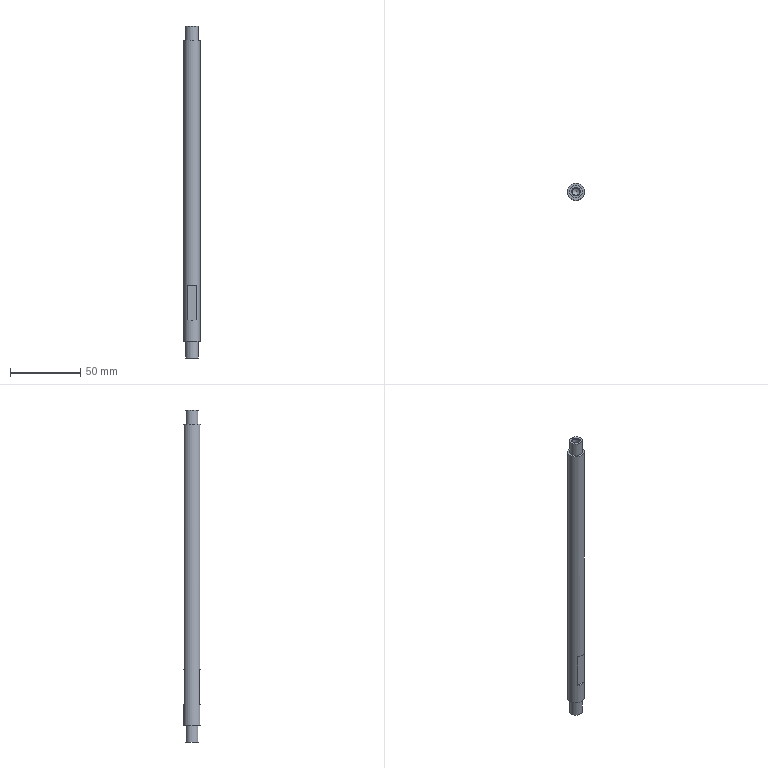Part | STEP file | YBQDJ-YY-10 | 1 solid | 19 faces | box 12 x 12 x 237 mm | volume 24995 mm3 | plane 10 | cylinder 5 | cone 4 | commonest cylinder face diameters 5 x2 9 x2 12 x1
STEP:
#1=CARTESIAN_POINT('',(0.,0.,0.));
#2=DIRECTION('',(0.,0.,1.));
#3=DIRECTION('',(1.,0.,0.));
#4=AXIS2_PLACEMENT_3D('',#1,#2,#3);
#5=CARTESIAN_POINT('',(260.5,385.,235.));
#6=VERTEX_POINT('',#5);
#7=CARTESIAN_POINT('',(266.5,385.,235.));
#8=DIRECTION('',(0.,0.,1.));
#9=DIRECTION('',(-1.,0.,0.));
#10=AXIS2_PLACEMENT_3D('',#7,#8,#9);
#11=CIRCLE('',#10,6.);
#12=CARTESIAN_POINT('',(266.5,385.,220.));
#13=DIRECTION('',(0.,0.,-1.));
#14=DIRECTION('',(1.,0.,0.));
#15=AXIS2_PLACEMENT_3D('',#12,#13,#14);
#16=CYLINDRICAL_SURFACE('',#15,6.);
#17=CARTESIAN_POINT('',(9.425,-15.));
#18=DIRECTION('',(-1.,0.));
#19=VECTOR('',#18,1.);
#20=LINE('',#17,#19);
#21=(GEOMETRIC_REPRESENTATION_CONTEXT(2)PARAMETRIC_REPRESENTATION_CONTEXT()REPRESENTATION_CONTEXT('',''));
#22=DEFINITIONAL_REPRESENTATION('',(#20),#21);
#23=PCURVE('',#16,#22);
#24=CARTESIAN_POINT('',(547.497,775.,235.));
#25=DIRECTION('',(0.,0.,1.));
#26=DIRECTION('',(-1.,0.,0.));
#27=AXIS2_PLACEMENT_3D('',#24,#25,#26);
#28=PLANE('',#27);
#29=CARTESIAN_POINT('',(280.997,390.));
#30=DIRECTION('',(1.,0.));
#31=AXIS2_PLACEMENT_2D('',#29,#30);
#32=CIRCLE('',#31,6.);
#33=(GEOMETRIC_REPRESENTATION_CONTEXT(2)PARAMETRIC_REPRESENTATION_CONTEXT()REPRESENTATION_CONTEXT('',''));
#34=DEFINITIONAL_REPRESENTATION('',(#32),#33);
#35=PCURVE('',#28,#34);
#36=SURFACE_CURVE('',#11,(#23,#35),.PCURVE_S1.);
#37=EDGE_CURVE('',#6,#6,#36,.T.);
#38=ORIENTED_EDGE('',*,*,#37,.F.);
#39=CARTESIAN_POINT('',(260.5,385.,20.));
#40=VERTEX_POINT('',#39);
#41=CARTESIAN_POINT('',(260.5,385.,235.));
#42=CARTESIAN_POINT('',(260.5,385.,20.));
#43=B_SPLINE_CURVE_WITH_KNOTS('',1,(#41,#42),.UNSPECIFIED.,.F.,.F.,(2,2),(-15.,200.),.PIECEWISE_BEZIER_KNOTS.);
#44=CARTESIAN_POINT('',(9.425,0.));
#45=DIRECTION('',(0.,1.));
#46=VECTOR('',#45,1.);
#47=LINE('',#44,#46);
#48=(GEOMETRIC_REPRESENTATION_CONTEXT(2)PARAMETRIC_REPRESENTATION_CONTEXT()REPRESENTATION_CONTEXT('',''));
#49=DEFINITIONAL_REPRESENTATION('',(#47),#48);
#50=PCURVE('',#16,#49);
#51=CARTESIAN_POINT('',(3.142,0.));
#52=DIRECTION('',(0.,1.));
#53=VECTOR('',#52,1.);
#54=LINE('',#51,#53);
#55=(GEOMETRIC_REPRESENTATION_CONTEXT(2)PARAMETRIC_REPRESENTATION_CONTEXT()REPRESENTATION_CONTEXT('',''));
#56=DEFINITIONAL_REPRESENTATION('',(#54),#55);
#57=PCURVE('',#16,#56);
#58=SEAM_CURVE('',#43,(#50,#57),.PCURVE_S1.);
#59=EDGE_CURVE('',#6,#40,#58,.T.);
#60=ORIENTED_EDGE('',*,*,#59,.T.);
#61=CARTESIAN_POINT('',(266.5,385.,20.));
#62=DIRECTION('',(0.,0.,1.));
#63=DIRECTION('',(-1.,0.,0.));
#64=AXIS2_PLACEMENT_3D('',#61,#62,#63);
#65=CIRCLE('',#64,6.);
#66=CARTESIAN_POINT('',(9.425,200.));
#67=DIRECTION('',(-1.,0.));
#68=VECTOR('',#67,1.);
#69=LINE('',#66,#68);
#70=(GEOMETRIC_REPRESENTATION_CONTEXT(2)PARAMETRIC_REPRESENTATION_CONTEXT()REPRESENTATION_CONTEXT('',''));
#71=DEFINITIONAL_REPRESENTATION('',(#69),#70);
#72=PCURVE('',#16,#71);
#73=CARTESIAN_POINT('',(266.5,385.,20.));
#74=DIRECTION('',(0.,0.,1.));
#75=DIRECTION('',(-1.,0.,0.));
#76=AXIS2_PLACEMENT_3D('',#73,#74,#75);
#77=PLANE('',#76);
#78=CARTESIAN_POINT('',(0.,0.));
#79=DIRECTION('',(1.,0.));
#80=AXIS2_PLACEMENT_2D('',#78,#79);
#81=CIRCLE('',#80,6.);
#82=(GEOMETRIC_REPRESENTATION_CONTEXT(2)PARAMETRIC_REPRESENTATION_CONTEXT()REPRESENTATION_CONTEXT('',''));
#83=DEFINITIONAL_REPRESENTATION('',(#81),#82);
#84=PCURVE('',#77,#83);
#85=SURFACE_CURVE('',#65,(#72,#84),.PCURVE_S1.);
#86=EDGE_CURVE('',#40,#40,#85,.T.);
#87=ORIENTED_EDGE('',*,*,#86,.T.);
#88=ORIENTED_EDGE('',*,*,#59,.F.);
#89=EDGE_LOOP('',(#38,#60,#87,#88));
#90=FACE_BOUND('',#89,.T.);
#91=CARTESIAN_POINT('',(263.183,390.,60.));
#92=VERTEX_POINT('',#91);
#93=CARTESIAN_POINT('',(269.817,390.,60.));
#94=VERTEX_POINT('',#93);
#95=CARTESIAN_POINT('',(266.5,385.,60.));
#96=DIRECTION('',(0.,0.,-1.));
#97=DIRECTION('',(0.,1.,0.));
#98=AXIS2_PLACEMENT_3D('',#95,#96,#97);
#99=CIRCLE('',#98,6.);
#100=CARTESIAN_POINT('',(-1.571,160.));
#101=DIRECTION('',(1.,0.));
#102=VECTOR('',#101,1.);
#103=LINE('',#100,#102);
#104=(GEOMETRIC_REPRESENTATION_CONTEXT(2)PARAMETRIC_REPRESENTATION_CONTEXT()REPRESENTATION_CONTEXT('',''));
#105=DEFINITIONAL_REPRESENTATION('',(#103),#104);
#106=PCURVE('',#16,#105);
#107=CARTESIAN_POINT('',(306.5,390.,60.));
#108=DIRECTION('',(0.,0.,-1.));
#109=DIRECTION('',(0.,1.,0.));
#110=AXIS2_PLACEMENT_3D('',#107,#108,#109);
#111=PLANE('',#110);
#112=CARTESIAN_POINT('',(-5.,-40.));
#113=DIRECTION('',(1.,0.));
#114=AXIS2_PLACEMENT_2D('',#112,#113);
#115=CIRCLE('',#114,6.);
#116=(GEOMETRIC_REPRESENTATION_CONTEXT(2)PARAMETRIC_REPRESENTATION_CONTEXT()REPRESENTATION_CONTEXT('',''));
#117=DEFINITIONAL_REPRESENTATION('',(#115),#116);
#118=PCURVE('',#111,#117);
#119=SURFACE_CURVE('',#99,(#106,#118),.PCURVE_S1.);
#120=EDGE_CURVE('',#92,#94,#119,.T.);
#121=ORIENTED_EDGE('',*,*,#120,.F.);
#122=CARTESIAN_POINT('',(263.183,390.,35.));
#123=VERTEX_POINT('',#122);
#124=CARTESIAN_POINT('',(263.183,390.,220.));
#125=DIRECTION('',(0.,0.,1.));
#126=VECTOR('',#125,1.);
#127=LINE('',#124,#126);
#128=CARTESIAN_POINT('',(4.127,0.));
#129=DIRECTION('',(0.,-1.));
#130=VECTOR('',#129,1.);
#131=LINE('',#128,#130);
#132=(GEOMETRIC_REPRESENTATION_CONTEXT(2)PARAMETRIC_REPRESENTATION_CONTEXT()REPRESENTATION_CONTEXT('',''));
#133=DEFINITIONAL_REPRESENTATION('',(#131),#132);
#134=PCURVE('',#16,#133);
#135=CARTESIAN_POINT('',(306.5,390.,35.));
#136=DIRECTION('',(0.,1.,0.));
#137=DIRECTION('',(0.,0.,1.));
#138=AXIS2_PLACEMENT_3D('',#135,#136,#137);
#139=PLANE('',#138);
#140=CARTESIAN_POINT('',(185.,-43.317));
#141=DIRECTION('',(1.,0.));
#142=VECTOR('',#141,1.);
#143=LINE('',#140,#142);
#144=(GEOMETRIC_REPRESENTATION_CONTEXT(2)PARAMETRIC_REPRESENTATION_CONTEXT()REPRESENTATION_CONTEXT('',''));
#145=DEFINITIONAL_REPRESENTATION('',(#143),#144);
#146=PCURVE('',#139,#145);
#147=SURFACE_CURVE('',#127,(#134,#146),.PCURVE_S1.);
#148=EDGE_CURVE('',#123,#92,#147,.T.);
#149=ORIENTED_EDGE('',*,*,#148,.F.);
#150=CARTESIAN_POINT('',(269.817,390.,35.));
#151=VERTEX_POINT('',#150);
#152=CARTESIAN_POINT('',(266.5,385.,35.));
#153=DIRECTION('',(0.,0.,1.));
#154=DIRECTION('',(0.,-1.,0.));
#155=AXIS2_PLACEMENT_3D('',#152,#153,#154);
#156=CIRCLE('',#155,6.);
#157=CARTESIAN_POINT('',(7.854,185.));
#158=DIRECTION('',(-1.,0.));
#159=VECTOR('',#158,1.);
#160=LINE('',#157,#159);
#161=(GEOMETRIC_REPRESENTATION_CONTEXT(2)PARAMETRIC_REPRESENTATION_CONTEXT()REPRESENTATION_CONTEXT('',''));
#162=DEFINITIONAL_REPRESENTATION('',(#160),#161);
#163=PCURVE('',#16,#162);
#164=CARTESIAN_POINT('',(306.5,406.,35.));
#165=DIRECTION('',(0.,0.,1.));
#166=DIRECTION('',(0.,-1.,0.));
#167=AXIS2_PLACEMENT_3D('',#164,#165,#166);
#168=PLANE('',#167);
#169=CARTESIAN_POINT('',(21.,-40.));
#170=DIRECTION('',(1.,0.));
#171=AXIS2_PLACEMENT_2D('',#169,#170);
#172=CIRCLE('',#171,6.);
#173=(GEOMETRIC_REPRESENTATION_CONTEXT(2)PARAMETRIC_REPRESENTATION_CONTEXT()REPRESENTATION_CONTEXT('',''));
#174=DEFINITIONAL_REPRESENTATION('',(#172),#173);
#175=PCURVE('',#168,#174);
#176=SURFACE_CURVE('',#156,(#163,#175),.PCURVE_S1.);
#177=EDGE_CURVE('',#151,#123,#176,.T.);
#178=ORIENTED_EDGE('',*,*,#177,.F.);
#179=CARTESIAN_POINT('',(269.817,390.,220.));
#180=DIRECTION('',(0.,0.,-1.));
#181=VECTOR('',#180,1.);
#182=LINE('',#179,#181);
#183=CARTESIAN_POINT('',(5.298,0.));
#184=DIRECTION('',(0.,1.));
#185=VECTOR('',#184,1.);
#186=LINE('',#183,#185);
#187=(GEOMETRIC_REPRESENTATION_CONTEXT(2)PARAMETRIC_REPRESENTATION_CONTEXT()REPRESENTATION_CONTEXT('',''));
#188=DEFINITIONAL_REPRESENTATION('',(#186),#187);
#189=PCURVE('',#16,#188);
#190=CARTESIAN_POINT('',(185.,-36.683));
#191=DIRECTION('',(-1.,0.));
#192=VECTOR('',#191,1.);
#193=LINE('',#190,#192);
#194=(GEOMETRIC_REPRESENTATION_CONTEXT(2)PARAMETRIC_REPRESENTATION_CONTEXT()REPRESENTATION_CONTEXT('',''));
#195=DEFINITIONAL_REPRESENTATION('',(#193),#194);
#196=PCURVE('',#139,#195);
#197=SURFACE_CURVE('',#182,(#189,#196),.PCURVE_S1.);
#198=EDGE_CURVE('',#94,#151,#197,.T.);
#199=ORIENTED_EDGE('',*,*,#198,.F.);
#200=EDGE_LOOP('',(#121,#149,#178,#199));
#201=FACE_BOUND('',#200,.T.);
#202=CARTESIAN_POINT('',(269.817,380.,60.));
#203=VERTEX_POINT('',#202);
#204=CARTESIAN_POINT('',(263.183,380.,60.));
#205=VERTEX_POINT('',#204);
#206=CARTESIAN_POINT('',(266.5,385.,60.));
#207=DIRECTION('',(0.,0.,-1.));
#208=DIRECTION('',(1.,0.,0.));
#209=AXIS2_PLACEMENT_3D('',#206,#207,#208);
#210=CIRCLE('',#209,6.);
#211=CARTESIAN_POINT('',(6.283,160.));
#212=DIRECTION('',(1.,0.));
#213=VECTOR('',#212,1.);
#214=LINE('',#211,#213);
#215=(GEOMETRIC_REPRESENTATION_CONTEXT(2)PARAMETRIC_REPRESENTATION_CONTEXT()REPRESENTATION_CONTEXT('',''));
#216=DEFINITIONAL_REPRESENTATION('',(#214),#215);
#217=PCURVE('',#16,#216);
#218=CARTESIAN_POINT('',(306.5,364.,60.));
#219=DIRECTION('',(0.,0.,-1.));
#220=DIRECTION('',(1.,0.,0.));
#221=AXIS2_PLACEMENT_3D('',#218,#219,#220);
#222=PLANE('',#221);
#223=CARTESIAN_POINT('',(-40.,-21.));
#224=DIRECTION('',(1.,0.));
#225=AXIS2_PLACEMENT_2D('',#223,#224);
#226=CIRCLE('',#225,6.);
#227=(GEOMETRIC_REPRESENTATION_CONTEXT(2)PARAMETRIC_REPRESENTATION_CONTEXT()REPRESENTATION_CONTEXT('',''));
#228=DEFINITIONAL_REPRESENTATION('',(#226),#227);
#229=PCURVE('',#222,#228);
#230=SURFACE_CURVE('',#210,(#217,#229),.PCURVE_S1.);
#231=EDGE_CURVE('',#203,#205,#230,.T.);
#232=ORIENTED_EDGE('',*,*,#231,.F.);
#233=CARTESIAN_POINT('',(269.817,380.,35.));
#234=VERTEX_POINT('',#233);
#235=CARTESIAN_POINT('',(269.817,380.,220.));
#236=DIRECTION('',(0.,0.,1.));
#237=VECTOR('',#236,1.);
#238=LINE('',#235,#237);
#239=CARTESIAN_POINT('',(7.268,0.));
#240=DIRECTION('',(0.,-1.));
#241=VECTOR('',#240,1.);
#242=LINE('',#239,#241);
#243=(GEOMETRIC_REPRESENTATION_CONTEXT(2)PARAMETRIC_REPRESENTATION_CONTEXT()REPRESENTATION_CONTEXT('',''));
#244=DEFINITIONAL_REPRESENTATION('',(#242),#243);
#245=PCURVE('',#16,#244);
#246=CARTESIAN_POINT('',(306.5,380.,60.));
#247=DIRECTION('',(0.,-1.,0.));
#248=DIRECTION('',(0.,0.,-1.));
#249=AXIS2_PLACEMENT_3D('',#246,#247,#248);
#250=PLANE('',#249);
#251=CARTESIAN_POINT('',(-160.,-36.683));
#252=DIRECTION('',(-1.,0.));
#253=VECTOR('',#252,1.);
#254=LINE('',#251,#253);
#255=(GEOMETRIC_REPRESENTATION_CONTEXT(2)PARAMETRIC_REPRESENTATION_CONTEXT()REPRESENTATION_CONTEXT('',''));
#256=DEFINITIONAL_REPRESENTATION('',(#254),#255);
#257=PCURVE('',#250,#256);
#258=SURFACE_CURVE('',#238,(#245,#257),.PCURVE_S1.);
#259=EDGE_CURVE('',#234,#203,#258,.T.);
#260=ORIENTED_EDGE('',*,*,#259,.F.);
#261=CARTESIAN_POINT('',(263.183,380.,35.));
#262=VERTEX_POINT('',#261);
#263=CARTESIAN_POINT('',(266.5,385.,35.));
#264=DIRECTION('',(0.,0.,1.));
#265=DIRECTION('',(0.,-1.,0.));
#266=AXIS2_PLACEMENT_3D('',#263,#264,#265);
#267=CIRCLE('',#266,6.);
#268=CARTESIAN_POINT('',(14.137,185.));
#269=DIRECTION('',(-1.,0.));
#270=VECTOR('',#269,1.);
#271=LINE('',#268,#270);
#272=(GEOMETRIC_REPRESENTATION_CONTEXT(2)PARAMETRIC_REPRESENTATION_CONTEXT()REPRESENTATION_CONTEXT('',''));
#273=DEFINITIONAL_REPRESENTATION('',(#271),#272);
#274=PCURVE('',#16,#273);
#275=CARTESIAN_POINT('',(306.5,380.,35.));
#276=DIRECTION('',(0.,0.,1.));
#277=DIRECTION('',(0.,-1.,0.));
#278=AXIS2_PLACEMENT_3D('',#275,#276,#277);
#279=PLANE('',#278);
#280=CARTESIAN_POINT('',(-5.,-40.));
#281=DIRECTION('',(1.,0.));
#282=AXIS2_PLACEMENT_2D('',#280,#281);
#283=CIRCLE('',#282,6.);
#284=(GEOMETRIC_REPRESENTATION_CONTEXT(2)PARAMETRIC_REPRESENTATION_CONTEXT()REPRESENTATION_CONTEXT('',''));
#285=DEFINITIONAL_REPRESENTATION('',(#283),#284);
#286=PCURVE('',#279,#285);
#287=SURFACE_CURVE('',#267,(#274,#286),.PCURVE_S1.);
#288=EDGE_CURVE('',#262,#234,#287,.T.);
#289=ORIENTED_EDGE('',*,*,#288,.F.);
#290=CARTESIAN_POINT('',(263.183,380.,220.));
#291=DIRECTION('',(0.,0.,-1.));
#292=VECTOR('',#291,1.);
#293=LINE('',#290,#292);
#294=CARTESIAN_POINT('',(8.44,0.));
#295=DIRECTION('',(0.,1.));
#296=VECTOR('',#295,1.);
#297=LINE('',#294,#296);
#298=(GEOMETRIC_REPRESENTATION_CONTEXT(2)PARAMETRIC_REPRESENTATION_CONTEXT()REPRESENTATION_CONTEXT('',''));
#299=DEFINITIONAL_REPRESENTATION('',(#297),#298);
#300=PCURVE('',#16,#299);
#301=CARTESIAN_POINT('',(-160.,-43.317));
#302=DIRECTION('',(1.,0.));
#303=VECTOR('',#302,1.);
#304=LINE('',#301,#303);
#305=(GEOMETRIC_REPRESENTATION_CONTEXT(2)PARAMETRIC_REPRESENTATION_CONTEXT()REPRESENTATION_CONTEXT('',''));
#306=DEFINITIONAL_REPRESENTATION('',(#304),#305);
#307=PCURVE('',#250,#306);
#308=SURFACE_CURVE('',#293,(#300,#307),.PCURVE_S1.);
#309=EDGE_CURVE('',#205,#262,#308,.T.);
#310=ORIENTED_EDGE('',*,*,#309,.F.);
#311=EDGE_LOOP('',(#232,#260,#289,#310));
#312=FACE_BOUND('',#311,.T.);
#313=ADVANCED_FACE('',(#90,#201,#312),#16,.T.);
#314=CARTESIAN_POINT('',(262.,385.,235.));
#315=VERTEX_POINT('',#314);
#316=CARTESIAN_POINT('',(266.5,385.,235.));
#317=DIRECTION('',(0.,0.,1.));
#318=DIRECTION('',(-1.,0.,0.));
#319=AXIS2_PLACEMENT_3D('',#316,#317,#318);
#320=CIRCLE('',#319,4.5);
#321=CARTESIAN_POINT('',(280.997,390.));
#322=DIRECTION('',(1.,0.));
#323=AXIS2_PLACEMENT_2D('',#321,#322);
#324=CIRCLE('',#323,4.5);
#325=(GEOMETRIC_REPRESENTATION_CONTEXT(2)PARAMETRIC_REPRESENTATION_CONTEXT()REPRESENTATION_CONTEXT('',''));
#326=DEFINITIONAL_REPRESENTATION('',(#324),#325);
#327=PCURVE('',#28,#326);
#328=CARTESIAN_POINT('',(266.5,385.,235.));
#329=DIRECTION('',(0.,0.,1.));
#330=DIRECTION('',(-1.,0.,0.));
#331=AXIS2_PLACEMENT_3D('',#328,#329,#330);
#332=CYLINDRICAL_SURFACE('',#331,4.5);
#333=CARTESIAN_POINT('',(0.,0.));
#334=DIRECTION('',(1.,0.));
#335=VECTOR('',#334,1.);
#336=LINE('',#333,#335);
#337=(GEOMETRIC_REPRESENTATION_CONTEXT(2)PARAMETRIC_REPRESENTATION_CONTEXT()REPRESENTATION_CONTEXT('',''));
#338=DEFINITIONAL_REPRESENTATION('',(#336),#337);
#339=PCURVE('',#332,#338);
#340=SURFACE_CURVE('',#320,(#327,#339),.PCURVE_S1.);
#341=EDGE_CURVE('',#315,#315,#340,.T.);
#342=ORIENTED_EDGE('',*,*,#341,.F.);
#343=EDGE_LOOP('',(#342));
#344=FACE_BOUND('',#343,.T.);
#345=ORIENTED_EDGE('',*,*,#37,.T.);
#346=EDGE_LOOP('',(#345));
#347=FACE_BOUND('',#346,.T.);
#348=ADVANCED_FACE('',(#344,#347),#28,.T.);
#349=CARTESIAN_POINT('',(262.,385.,20.));
#350=VERTEX_POINT('',#349);
#351=CARTESIAN_POINT('',(266.5,385.,20.));
#352=DIRECTION('',(0.,0.,1.));
#353=DIRECTION('',(-1.,0.,0.));
#354=AXIS2_PLACEMENT_3D('',#351,#352,#353);
#355=CIRCLE('',#354,4.5);
#356=CARTESIAN_POINT('',(0.,0.));
#357=DIRECTION('',(1.,0.));
#358=AXIS2_PLACEMENT_2D('',#356,#357);
#359=CIRCLE('',#358,4.5);
#360=(GEOMETRIC_REPRESENTATION_CONTEXT(2)PARAMETRIC_REPRESENTATION_CONTEXT()REPRESENTATION_CONTEXT('',''));
#361=DEFINITIONAL_REPRESENTATION('',(#359),#360);
#362=PCURVE('',#77,#361);
#363=CARTESIAN_POINT('',(266.5,385.,20.));
#364=DIRECTION('',(0.,0.,-1.));
#365=DIRECTION('',(1.,0.,0.));
#366=AXIS2_PLACEMENT_3D('',#363,#364,#365);
#367=CYLINDRICAL_SURFACE('',#366,4.5);
#368=CARTESIAN_POINT('',(9.425,0.));
#369=DIRECTION('',(-1.,0.));
#370=VECTOR('',#369,1.);
#371=LINE('',#368,#370);
#372=(GEOMETRIC_REPRESENTATION_CONTEXT(2)PARAMETRIC_REPRESENTATION_CONTEXT()REPRESENTATION_CONTEXT('',''));
#373=DEFINITIONAL_REPRESENTATION('',(#371),#372);
#374=PCURVE('',#367,#373);
#375=SURFACE_CURVE('',#355,(#362,#374),.PCURVE_S1.);
#376=EDGE_CURVE('',#350,#350,#375,.T.);
#377=ORIENTED_EDGE('',*,*,#376,.T.);
#378=EDGE_LOOP('',(#377));
#379=FACE_BOUND('',#378,.T.);
#380=ORIENTED_EDGE('',*,*,#86,.F.);
#381=EDGE_LOOP('',(#380));
#382=FACE_BOUND('',#381,.T.);
#383=ADVANCED_FACE('',(#379,#382),#77,.F.);
#384=ORIENTED_EDGE('',*,*,#341,.T.);
#385=CARTESIAN_POINT('',(262.,385.,245.));
#386=VERTEX_POINT('',#385);
#387=CARTESIAN_POINT('',(262.,385.,235.));
#388=CARTESIAN_POINT('',(262.,385.,245.));
#389=B_SPLINE_CURVE_WITH_KNOTS('',1,(#387,#388),.UNSPECIFIED.,.F.,.F.,(2,2),(0.,10.),.PIECEWISE_BEZIER_KNOTS.);
#390=CARTESIAN_POINT('',(6.283,0.));
#391=DIRECTION('',(0.,1.));
#392=VECTOR('',#391,1.);
#393=LINE('',#390,#392);
#394=(GEOMETRIC_REPRESENTATION_CONTEXT(2)PARAMETRIC_REPRESENTATION_CONTEXT()REPRESENTATION_CONTEXT('',''));
#395=DEFINITIONAL_REPRESENTATION('',(#393),#394);
#396=PCURVE('',#332,#395);
#397=CARTESIAN_POINT('',(0.,0.));
#398=DIRECTION('',(0.,1.));
#399=VECTOR('',#398,1.);
#400=LINE('',#397,#399);
#401=(GEOMETRIC_REPRESENTATION_CONTEXT(2)PARAMETRIC_REPRESENTATION_CONTEXT()REPRESENTATION_CONTEXT('',''));
#402=DEFINITIONAL_REPRESENTATION('',(#400),#401);
#403=PCURVE('',#332,#402);
#404=SEAM_CURVE('',#389,(#396,#403),.PCURVE_S1.);
#405=EDGE_CURVE('',#315,#386,#404,.T.);
#406=ORIENTED_EDGE('',*,*,#405,.T.);
#407=CARTESIAN_POINT('',(266.5,385.,245.));
#408=DIRECTION('',(0.,0.,1.));
#409=DIRECTION('',(-1.,0.,0.));
#410=AXIS2_PLACEMENT_3D('',#407,#408,#409);
#411=CIRCLE('',#410,4.5);
#412=CARTESIAN_POINT('',(0.,10.));
#413=DIRECTION('',(1.,0.));
#414=VECTOR('',#413,1.);
#415=LINE('',#412,#414);
#416=(GEOMETRIC_REPRESENTATION_CONTEXT(2)PARAMETRIC_REPRESENTATION_CONTEXT()REPRESENTATION_CONTEXT('',''));
#417=DEFINITIONAL_REPRESENTATION('',(#415),#416);
#418=PCURVE('',#332,#417);
#419=CARTESIAN_POINT('',(266.5,385.,245.));
#420=DIRECTION('',(0.,0.,1.));
#421=DIRECTION('',(-1.,0.,0.));
#422=AXIS2_PLACEMENT_3D('',#419,#420,#421);
#423=PLANE('',#422);
#424=CARTESIAN_POINT('',(0.,0.));
#425=DIRECTION('',(1.,0.));
#426=AXIS2_PLACEMENT_2D('',#424,#425);
#427=CIRCLE('',#426,4.5);
#428=(GEOMETRIC_REPRESENTATION_CONTEXT(2)PARAMETRIC_REPRESENTATION_CONTEXT()REPRESENTATION_CONTEXT('',''));
#429=DEFINITIONAL_REPRESENTATION('',(#427),#428);
#430=PCURVE('',#423,#429);
#431=SURFACE_CURVE('',#411,(#418,#430),.PCURVE_S1.);
#432=EDGE_CURVE('',#386,#386,#431,.T.);
#433=ORIENTED_EDGE('',*,*,#432,.F.);
#434=ORIENTED_EDGE('',*,*,#405,.F.);
#435=EDGE_LOOP('',(#384,#406,#433,#434));
#436=FACE_BOUND('',#435,.T.);
#437=ADVANCED_FACE('',(#436),#332,.T.);
#438=CARTESIAN_POINT('',(263.5,385.,245.));
#439=VERTEX_POINT('',#438);
#440=CARTESIAN_POINT('',(266.5,385.,245.));
#441=DIRECTION('',(0.,0.,-1.));
#442=DIRECTION('',(-1.,0.,0.));
#443=AXIS2_PLACEMENT_3D('',#440,#441,#442);
#444=CIRCLE('',#443,3.);
#445=CARTESIAN_POINT('',(3.,0.));
#446=CARTESIAN_POINT('',(3.,-5.196));
#447=CARTESIAN_POINT('',(-1.5,-2.598));
#448=CARTESIAN_POINT('',(-6.,0.));
#449=CARTESIAN_POINT('',(-1.5,2.598));
#450=CARTESIAN_POINT('',(3.,5.196));
#451=CARTESIAN_POINT('',(3.,0.));
#452=(BOUNDED_CURVE()B_SPLINE_CURVE(2,(#445,#446,#447,#448,#449,#450,#451),.UNSPECIFIED.,.T.,.F.)B_SPLINE_CURVE_WITH_KNOTS((1,2,2,2,2,1),(-2.094,0.,2.094,4.189,6.283,8.378),.UNSPECIFIED.)CURVE()GEOMETRIC_REPRESENTATION_ITEM()RATIONAL_B_SPLINE_CURVE((1.,0.5,1.,0.5,1.,0.5,1.))REPRESENTATION_ITEM(''));
#453=(GEOMETRIC_REPRESENTATION_CONTEXT(2)PARAMETRIC_REPRESENTATION_CONTEXT()REPRESENTATION_CONTEXT('',''));
#454=DEFINITIONAL_REPRESENTATION('',(#452),#453);
#455=PCURVE('',#423,#454);
#456=CARTESIAN_POINT('',(266.5,385.,245.));
#457=DIRECTION('',(0.,0.,1.));
#458=DIRECTION('',(-1.,0.,0.));
#459=AXIS2_PLACEMENT_3D('',#456,#457,#458);
#460=CONICAL_SURFACE('',#459,3.,0.7854);
#461=CARTESIAN_POINT('',(6.283,0.));
#462=DIRECTION('',(-1.,0.));
#463=VECTOR('',#462,1.);
#464=LINE('',#461,#463);
#465=(GEOMETRIC_REPRESENTATION_CONTEXT(2)PARAMETRIC_REPRESENTATION_CONTEXT()REPRESENTATION_CONTEXT('',''));
#466=DEFINITIONAL_REPRESENTATION('',(#464),#465);
#467=PCURVE('',#460,#466);
#468=SURFACE_CURVE('',#444,(#455,#467),.PCURVE_S1.);
#469=EDGE_CURVE('',#439,#439,#468,.T.);
#470=ORIENTED_EDGE('',*,*,#469,.T.);
#471=EDGE_LOOP('',(#470));
#472=FACE_BOUND('',#471,.T.);
#473=ORIENTED_EDGE('',*,*,#432,.T.);
#474=EDGE_LOOP('',(#473));
#475=FACE_BOUND('',#474,.T.);
#476=ADVANCED_FACE('',(#472,#475),#423,.T.);
#477=ORIENTED_EDGE('',*,*,#376,.F.);
#478=CARTESIAN_POINT('',(262.,385.,8.));
#479=VERTEX_POINT('',#478);
#480=CARTESIAN_POINT('',(262.,385.,20.));
#481=CARTESIAN_POINT('',(262.,385.,8.));
#482=B_SPLINE_CURVE_WITH_KNOTS('',1,(#480,#481),.UNSPECIFIED.,.F.,.F.,(2,2),(0.,12.),.PIECEWISE_BEZIER_KNOTS.);
#483=CARTESIAN_POINT('',(9.425,0.));
#484=DIRECTION('',(0.,1.));
#485=VECTOR('',#484,1.);
#486=LINE('',#483,#485);
#487=(GEOMETRIC_REPRESENTATION_CONTEXT(2)PARAMETRIC_REPRESENTATION_CONTEXT()REPRESENTATION_CONTEXT('',''));
#488=DEFINITIONAL_REPRESENTATION('',(#486),#487);
#489=PCURVE('',#367,#488);
#490=CARTESIAN_POINT('',(3.142,0.));
#491=DIRECTION('',(0.,1.));
#492=VECTOR('',#491,1.);
#493=LINE('',#490,#492);
#494=(GEOMETRIC_REPRESENTATION_CONTEXT(2)PARAMETRIC_REPRESENTATION_CONTEXT()REPRESENTATION_CONTEXT('',''));
#495=DEFINITIONAL_REPRESENTATION('',(#493),#494);
#496=PCURVE('',#367,#495);
#497=SEAM_CURVE('',#482,(#489,#496),.PCURVE_S1.);
#498=EDGE_CURVE('',#350,#479,#497,.T.);
#499=ORIENTED_EDGE('',*,*,#498,.T.);
#500=CARTESIAN_POINT('',(266.5,385.,8.));
#501=DIRECTION('',(0.,0.,1.));
#502=DIRECTION('',(-1.,0.,0.));
#503=AXIS2_PLACEMENT_3D('',#500,#501,#502);
#504=CIRCLE('',#503,4.5);
#505=CARTESIAN_POINT('',(9.425,12.));
#506=DIRECTION('',(-1.,0.));
#507=VECTOR('',#506,1.);
#508=LINE('',#505,#507);
#509=(GEOMETRIC_REPRESENTATION_CONTEXT(2)PARAMETRIC_REPRESENTATION_CONTEXT()REPRESENTATION_CONTEXT('',''));
#510=DEFINITIONAL_REPRESENTATION('',(#508),#509);
#511=PCURVE('',#367,#510);
#512=CARTESIAN_POINT('',(266.5,385.,8.));
#513=DIRECTION('',(0.,0.,1.));
#514=DIRECTION('',(-1.,0.,0.));
#515=AXIS2_PLACEMENT_3D('',#512,#513,#514);
#516=PLANE('',#515);
#517=CARTESIAN_POINT('',(0.,0.));
#518=DIRECTION('',(1.,0.));
#519=AXIS2_PLACEMENT_2D('',#517,#518);
#520=CIRCLE('',#519,4.5);
#521=(GEOMETRIC_REPRESENTATION_CONTEXT(2)PARAMETRIC_REPRESENTATION_CONTEXT()REPRESENTATION_CONTEXT('',''));
#522=DEFINITIONAL_REPRESENTATION('',(#520),#521);
#523=PCURVE('',#516,#522);
#524=SURFACE_CURVE('',#504,(#511,#523),.PCURVE_S1.);
#525=EDGE_CURVE('',#479,#479,#524,.T.);
#526=ORIENTED_EDGE('',*,*,#525,.T.);
#527=ORIENTED_EDGE('',*,*,#498,.F.);
#528=EDGE_LOOP('',(#477,#499,#526,#527));
#529=FACE_BOUND('',#528,.T.);
#530=ADVANCED_FACE('',(#529),#367,.T.);
#531=CARTESIAN_POINT('',(263.5,385.,8.));
#532=VERTEX_POINT('',#531);
#533=CARTESIAN_POINT('',(266.5,385.,8.));
#534=DIRECTION('',(0.,0.,1.));
#535=DIRECTION('',(-1.,0.,0.));
#536=AXIS2_PLACEMENT_3D('',#533,#534,#535);
#537=CIRCLE('',#536,3.);
#538=CARTESIAN_POINT('',(0.,0.));
#539=DIRECTION('',(1.,0.));
#540=AXIS2_PLACEMENT_2D('',#538,#539);
#541=CIRCLE('',#540,3.);
#542=(GEOMETRIC_REPRESENTATION_CONTEXT(2)PARAMETRIC_REPRESENTATION_CONTEXT()REPRESENTATION_CONTEXT('',''));
#543=DEFINITIONAL_REPRESENTATION('',(#541),#542);
#544=PCURVE('',#516,#543);
#545=CARTESIAN_POINT('',(266.5,385.,8.));
#546=DIRECTION('',(0.,0.,-1.));
#547=DIRECTION('',(1.,0.,0.));
#548=AXIS2_PLACEMENT_3D('',#545,#546,#547);
#549=CONICAL_SURFACE('',#548,3.,0.7854);
#550=CARTESIAN_POINT('',(9.425,0.));
#551=DIRECTION('',(-1.,0.));
#552=VECTOR('',#551,1.);
#553=LINE('',#550,#552);
#554=(GEOMETRIC_REPRESENTATION_CONTEXT(2)PARAMETRIC_REPRESENTATION_CONTEXT()REPRESENTATION_CONTEXT('',''));
#555=DEFINITIONAL_REPRESENTATION('',(#553),#554);
#556=PCURVE('',#549,#555);
#557=SURFACE_CURVE('',#537,(#544,#556),.PCURVE_S1.);
#558=EDGE_CURVE('',#532,#532,#557,.T.);
#559=ORIENTED_EDGE('',*,*,#558,.T.);
#560=EDGE_LOOP('',(#559));
#561=FACE_BOUND('',#560,.T.);
#562=ORIENTED_EDGE('',*,*,#525,.F.);
#563=EDGE_LOOP('',(#562));
#564=FACE_BOUND('',#563,.T.);
#565=ADVANCED_FACE('',(#561,#564),#516,.F.);
#566=CARTESIAN_POINT('',(264.,385.,233.));
#567=VERTEX_POINT('',#566);
#568=CARTESIAN_POINT('',(269.,385.,233.));
#569=VERTEX_POINT('',#568);
#570=CARTESIAN_POINT('',(266.5,385.,233.));
#571=DIRECTION('',(0.,0.,1.));
#572=DIRECTION('',(1.,0.,0.));
#573=AXIS2_PLACEMENT_3D('',#570,#571,#572);
#574=CIRCLE('',#573,2.5);
#575=CARTESIAN_POINT('',(266.5,385.,233.));
#576=DIRECTION('',(0.,0.,1.));
#577=DIRECTION('',(-1.,0.,0.));
#578=AXIS2_PLACEMENT_3D('',#575,#576,#577);
#579=CONICAL_SURFACE('',#578,2.5,1.03);
#580=CARTESIAN_POINT('',(-3.142,0.));
#581=DIRECTION('',(1.,0.));
#582=VECTOR('',#581,1.);
#583=LINE('',#580,#582);
#584=(GEOMETRIC_REPRESENTATION_CONTEXT(2)PARAMETRIC_REPRESENTATION_CONTEXT()REPRESENTATION_CONTEXT('',''));
#585=DEFINITIONAL_REPRESENTATION('',(#583),#584);
#586=PCURVE('',#579,#585);
#587=CARTESIAN_POINT('',(266.5,385.,245.));
#588=DIRECTION('',(0.,0.,-1.));
#589=DIRECTION('',(1.,0.,0.));
#590=AXIS2_PLACEMENT_3D('',#587,#588,#589);
#591=CYLINDRICAL_SURFACE('',#590,2.5);
#592=CARTESIAN_POINT('',(12.566,12.));
#593=DIRECTION('',(-1.,0.));
#594=VECTOR('',#593,1.);
#595=LINE('',#592,#594);
#596=(GEOMETRIC_REPRESENTATION_CONTEXT(2)PARAMETRIC_REPRESENTATION_CONTEXT()REPRESENTATION_CONTEXT('',''));
#597=DEFINITIONAL_REPRESENTATION('',(#595),#596);
#598=PCURVE('',#591,#597);
#599=SURFACE_CURVE('',#574,(#586,#598),.PCURVE_S1.);
#600=EDGE_CURVE('',#567,#569,#599,.T.);
#601=ORIENTED_EDGE('',*,*,#600,.F.);
#602=CARTESIAN_POINT('',(266.5,385.,231.498));
#603=VERTEX_POINT('',#602);
#604=CARTESIAN_POINT('',(266.5,385.,231.498));
#605=CARTESIAN_POINT('',(264.,385.,233.));
#606=B_SPLINE_CURVE_WITH_KNOTS('',1,(#604,#605),.UNSPECIFIED.,.F.,.F.,(2,2),(-2.917,0.),.PIECEWISE_BEZIER_KNOTS.);
#607=CARTESIAN_POINT('',(0.,0.));
#608=DIRECTION('',(0.,1.));
#609=VECTOR('',#608,1.);
#610=LINE('',#607,#609);
#611=(GEOMETRIC_REPRESENTATION_CONTEXT(2)PARAMETRIC_REPRESENTATION_CONTEXT()REPRESENTATION_CONTEXT('',''));
#612=DEFINITIONAL_REPRESENTATION('',(#610),#611);
#613=PCURVE('',#579,#612);
#614=CARTESIAN_POINT('',(6.283,0.));
#615=DIRECTION('',(0.,1.));
#616=VECTOR('',#615,1.);
#617=LINE('',#614,#616);
#618=(GEOMETRIC_REPRESENTATION_CONTEXT(2)PARAMETRIC_REPRESENTATION_CONTEXT()REPRESENTATION_CONTEXT('',''));
#619=DEFINITIONAL_REPRESENTATION('',(#617),#618);
#620=PCURVE('',#579,#619);
#621=SEAM_CURVE('',#606,(#613,#620),.PCURVE_S1.);
#622=EDGE_CURVE('',#603,#567,#621,.T.);
#623=ORIENTED_EDGE('',*,*,#622,.F.);
#624=ORIENTED_EDGE('',*,*,#622,.T.);
#625=CARTESIAN_POINT('',(266.5,385.,233.));
#626=DIRECTION('',(0.,0.,1.));
#627=DIRECTION('',(1.,0.,0.));
#628=AXIS2_PLACEMENT_3D('',#625,#626,#627);
#629=CIRCLE('',#628,2.5);
#630=CARTESIAN_POINT('',(3.142,0.));
#631=DIRECTION('',(1.,0.));
#632=VECTOR('',#631,1.);
#633=LINE('',#630,#632);
#634=(GEOMETRIC_REPRESENTATION_CONTEXT(2)PARAMETRIC_REPRESENTATION_CONTEXT()REPRESENTATION_CONTEXT('',''));
#635=DEFINITIONAL_REPRESENTATION('',(#633),#634);
#636=PCURVE('',#579,#635);
#637=CARTESIAN_POINT('',(6.283,12.));
#638=DIRECTION('',(-1.,0.));
#639=VECTOR('',#638,1.);
#640=LINE('',#637,#639);
#641=(GEOMETRIC_REPRESENTATION_CONTEXT(2)PARAMETRIC_REPRESENTATION_CONTEXT()REPRESENTATION_CONTEXT('',''));
#642=DEFINITIONAL_REPRESENTATION('',(#640),#641);
#643=PCURVE('',#591,#642);
#644=SURFACE_CURVE('',#629,(#636,#643),.PCURVE_S1.);
#645=EDGE_CURVE('',#569,#567,#644,.T.);
#646=ORIENTED_EDGE('',*,*,#645,.F.);
#647=EDGE_LOOP('',(#601,#623,#624,#646));
#648=FACE_BOUND('',#647,.F.);
#649=ADVANCED_FACE('',(#648),#579,.F.);
#650=CARTESIAN_POINT('',(264.,385.,244.5));
#651=VERTEX_POINT('',#650);
#652=CARTESIAN_POINT('',(266.5,385.,244.5));
#653=DIRECTION('',(0.,0.,1.));
#654=DIRECTION('',(-1.,0.,0.));
#655=AXIS2_PLACEMENT_3D('',#652,#653,#654);
#656=CIRCLE('',#655,2.5);
#657=CARTESIAN_POINT('',(9.425,0.5));
#658=DIRECTION('',(-1.,0.));
#659=VECTOR('',#658,1.);
#660=LINE('',#657,#659);
#661=(GEOMETRIC_REPRESENTATION_CONTEXT(2)PARAMETRIC_REPRESENTATION_CONTEXT()REPRESENTATION_CONTEXT('',''));
#662=DEFINITIONAL_REPRESENTATION('',(#660),#661);
#663=PCURVE('',#591,#662);
#664=CARTESIAN_POINT('',(0.,-0.5));
#665=DIRECTION('',(1.,0.));
#666=VECTOR('',#665,1.);
#667=LINE('',#664,#666);
#668=(GEOMETRIC_REPRESENTATION_CONTEXT(2)PARAMETRIC_REPRESENTATION_CONTEXT()REPRESENTATION_CONTEXT('',''));
#669=DEFINITIONAL_REPRESENTATION('',(#667),#668);
#670=PCURVE('',#460,#669);
#671=SURFACE_CURVE('',#656,(#663,#670),.PCURVE_S1.);
#672=EDGE_CURVE('',#651,#651,#671,.T.);
#673=ORIENTED_EDGE('',*,*,#672,.F.);
#674=CARTESIAN_POINT('',(264.,385.,244.5));
#675=CARTESIAN_POINT('',(264.,385.,233.));
#676=B_SPLINE_CURVE_WITH_KNOTS('',1,(#674,#675),.UNSPECIFIED.,.F.,.F.,(2,2),(0.5,12.),.PIECEWISE_BEZIER_KNOTS.);
#677=CARTESIAN_POINT('',(9.425,0.));
#678=DIRECTION('',(0.,1.));
#679=VECTOR('',#678,1.);
#680=LINE('',#677,#679);
#681=(GEOMETRIC_REPRESENTATION_CONTEXT(2)PARAMETRIC_REPRESENTATION_CONTEXT()REPRESENTATION_CONTEXT('',''));
#682=DEFINITIONAL_REPRESENTATION('',(#680),#681);
#683=PCURVE('',#591,#682);
#684=CARTESIAN_POINT('',(3.142,0.));
#685=DIRECTION('',(0.,1.));
#686=VECTOR('',#685,1.);
#687=LINE('',#684,#686);
#688=(GEOMETRIC_REPRESENTATION_CONTEXT(2)PARAMETRIC_REPRESENTATION_CONTEXT()REPRESENTATION_CONTEXT('',''));
#689=DEFINITIONAL_REPRESENTATION('',(#687),#688);
#690=PCURVE('',#591,#689);
#691=SEAM_CURVE('',#676,(#683,#690),.PCURVE_S1.);
#692=EDGE_CURVE('',#651,#567,#691,.T.);
#693=ORIENTED_EDGE('',*,*,#692,.T.);
#694=ORIENTED_EDGE('',*,*,#600,.T.);
#695=ORIENTED_EDGE('',*,*,#645,.T.);
#696=ORIENTED_EDGE('',*,*,#692,.F.);
#697=EDGE_LOOP('',(#673,#693,#694,#695,#696));
#698=FACE_BOUND('',#697,.F.);
#699=ADVANCED_FACE('',(#698),#591,.F.);
#700=ORIENTED_EDGE('',*,*,#672,.T.);
#701=CARTESIAN_POINT('',(264.,385.,244.5));
#702=CARTESIAN_POINT('',(263.5,385.,245.));
#703=B_SPLINE_CURVE_WITH_KNOTS('',1,(#701,#702),.UNSPECIFIED.,.F.,.F.,(2,2),(-0.7071,0.),.PIECEWISE_BEZIER_KNOTS.);
#704=CARTESIAN_POINT('',(6.283,0.));
#705=DIRECTION('',(0.,1.));
#706=VECTOR('',#705,1.);
#707=LINE('',#704,#706);
#708=(GEOMETRIC_REPRESENTATION_CONTEXT(2)PARAMETRIC_REPRESENTATION_CONTEXT()REPRESENTATION_CONTEXT('',''));
#709=DEFINITIONAL_REPRESENTATION('',(#707),#708);
#710=PCURVE('',#460,#709);
#711=CARTESIAN_POINT('',(0.,0.));
#712=DIRECTION('',(0.,1.));
#713=VECTOR('',#712,1.);
#714=LINE('',#711,#713);
#715=(GEOMETRIC_REPRESENTATION_CONTEXT(2)PARAMETRIC_REPRESENTATION_CONTEXT()REPRESENTATION_CONTEXT('',''));
#716=DEFINITIONAL_REPRESENTATION('',(#714),#715);
#717=PCURVE('',#460,#716);
#718=SEAM_CURVE('',#703,(#710,#717),.PCURVE_S1.);
#719=EDGE_CURVE('',#651,#439,#718,.T.);
#720=ORIENTED_EDGE('',*,*,#719,.T.);
#721=ORIENTED_EDGE('',*,*,#469,.T.);
#722=ORIENTED_EDGE('',*,*,#719,.F.);
#723=EDGE_LOOP('',(#700,#720,#721,#722));
#724=FACE_BOUND('',#723,.F.);
#725=ADVANCED_FACE('',(#724),#460,.F.);
#726=CARTESIAN_POINT('',(269.,385.,20.));
#727=VERTEX_POINT('',#726);
#728=CARTESIAN_POINT('',(264.,385.,20.));
#729=VERTEX_POINT('',#728);
#730=CARTESIAN_POINT('',(266.5,385.,20.));
#731=DIRECTION('',(0.,0.,-1.));
#732=DIRECTION('',(-1.,0.,0.));
#733=AXIS2_PLACEMENT_3D('',#730,#731,#732);
#734=CIRCLE('',#733,2.5);
#735=CARTESIAN_POINT('',(266.5,385.,20.));
#736=DIRECTION('',(0.,0.,-1.));
#737=DIRECTION('',(1.,0.,0.));
#738=AXIS2_PLACEMENT_3D('',#735,#736,#737);
#739=CONICAL_SURFACE('',#738,2.5,1.03);
#740=CARTESIAN_POINT('',(-3.142,0.));
#741=DIRECTION('',(1.,0.));
#742=VECTOR('',#741,1.);
#743=LINE('',#740,#742);
#744=(GEOMETRIC_REPRESENTATION_CONTEXT(2)PARAMETRIC_REPRESENTATION_CONTEXT()REPRESENTATION_CONTEXT('',''));
#745=DEFINITIONAL_REPRESENTATION('',(#743),#744);
#746=PCURVE('',#739,#745);
#747=CARTESIAN_POINT('',(266.5,385.,8.));
#748=DIRECTION('',(0.,0.,1.));
#749=DIRECTION('',(-1.,0.,0.));
#750=AXIS2_PLACEMENT_3D('',#747,#748,#749);
#751=CYLINDRICAL_SURFACE('',#750,2.5);
#752=CARTESIAN_POINT('',(6.283,12.));
#753=DIRECTION('',(-1.,0.));
#754=VECTOR('',#753,1.);
#755=LINE('',#752,#754);
#756=(GEOMETRIC_REPRESENTATION_CONTEXT(2)PARAMETRIC_REPRESENTATION_CONTEXT()REPRESENTATION_CONTEXT('',''));
#757=DEFINITIONAL_REPRESENTATION('',(#755),#756);
#758=PCURVE('',#751,#757);
#759=SURFACE_CURVE('',#734,(#746,#758),.PCURVE_S1.);
#760=EDGE_CURVE('',#727,#729,#759,.T.);
#761=ORIENTED_EDGE('',*,*,#760,.F.);
#762=CARTESIAN_POINT('',(266.5,385.,21.502));
#763=VERTEX_POINT('',#762);
#764=CARTESIAN_POINT('',(266.5,385.,21.502));
#765=CARTESIAN_POINT('',(269.,385.,20.));
#766=B_SPLINE_CURVE_WITH_KNOTS('',1,(#764,#765),.UNSPECIFIED.,.F.,.F.,(2,2),(-2.917,0.),.PIECEWISE_BEZIER_KNOTS.);
#767=CARTESIAN_POINT('',(0.,0.));
#768=DIRECTION('',(0.,1.));
#769=VECTOR('',#768,1.);
#770=LINE('',#767,#769);
#771=(GEOMETRIC_REPRESENTATION_CONTEXT(2)PARAMETRIC_REPRESENTATION_CONTEXT()REPRESENTATION_CONTEXT('',''));
#772=DEFINITIONAL_REPRESENTATION('',(#770),#771);
#773=PCURVE('',#739,#772);
#774=CARTESIAN_POINT('',(6.283,0.));
#775=DIRECTION('',(0.,1.));
#776=VECTOR('',#775,1.);
#777=LINE('',#774,#776);
#778=(GEOMETRIC_REPRESENTATION_CONTEXT(2)PARAMETRIC_REPRESENTATION_CONTEXT()REPRESENTATION_CONTEXT('',''));
#779=DEFINITIONAL_REPRESENTATION('',(#777),#778);
#780=PCURVE('',#739,#779);
#781=SEAM_CURVE('',#766,(#773,#780),.PCURVE_S1.);
#782=EDGE_CURVE('',#763,#727,#781,.T.);
#783=ORIENTED_EDGE('',*,*,#782,.F.);
#784=ORIENTED_EDGE('',*,*,#782,.T.);
#785=CARTESIAN_POINT('',(266.5,385.,20.));
#786=DIRECTION('',(0.,0.,-1.));
#787=DIRECTION('',(-1.,0.,0.));
#788=AXIS2_PLACEMENT_3D('',#785,#786,#787);
#789=CIRCLE('',#788,2.5);
#790=CARTESIAN_POINT('',(3.142,0.));
#791=DIRECTION('',(1.,0.));
#792=VECTOR('',#791,1.);
#793=LINE('',#790,#792);
#794=(GEOMETRIC_REPRESENTATION_CONTEXT(2)PARAMETRIC_REPRESENTATION_CONTEXT()REPRESENTATION_CONTEXT('',''));
#795=DEFINITIONAL_REPRESENTATION('',(#793),#794);
#796=PCURVE('',#739,#795);
#797=CARTESIAN_POINT('',(6.283,12.));
#798=DIRECTION('',(-1.,0.));
#799=VECTOR('',#798,1.);
#800=LINE('',#797,#799);
#801=(GEOMETRIC_REPRESENTATION_CONTEXT(2)PARAMETRIC_REPRESENTATION_CONTEXT()REPRESENTATION_CONTEXT('',''));
#802=DEFINITIONAL_REPRESENTATION('',(#800),#801);
#803=PCURVE('',#751,#802);
#804=SURFACE_CURVE('',#789,(#796,#803),.PCURVE_S1.);
#805=EDGE_CURVE('',#729,#727,#804,.T.);
#806=ORIENTED_EDGE('',*,*,#805,.F.);
#807=EDGE_LOOP('',(#761,#783,#784,#806));
#808=FACE_BOUND('',#807,.F.);
#809=ADVANCED_FACE('',(#808),#739,.F.);
#810=CARTESIAN_POINT('',(264.,385.,8.5));
#811=VERTEX_POINT('',#810);
#812=CARTESIAN_POINT('',(266.5,385.,8.5));
#813=DIRECTION('',(0.,0.,-1.));
#814=DIRECTION('',(-1.,0.,0.));
#815=AXIS2_PLACEMENT_3D('',#812,#813,#814);
#816=CIRCLE('',#815,2.5);
#817=CARTESIAN_POINT('',(6.283,0.5));
#818=DIRECTION('',(-1.,0.));
#819=VECTOR('',#818,1.);
#820=LINE('',#817,#819);
#821=(GEOMETRIC_REPRESENTATION_CONTEXT(2)PARAMETRIC_REPRESENTATION_CONTEXT()REPRESENTATION_CONTEXT('',''));
#822=DEFINITIONAL_REPRESENTATION('',(#820),#821);
#823=PCURVE('',#751,#822);
#824=CARTESIAN_POINT('',(3.142,-0.5));
#825=DIRECTION('',(1.,0.));
#826=VECTOR('',#825,1.);
#827=LINE('',#824,#826);
#828=(GEOMETRIC_REPRESENTATION_CONTEXT(2)PARAMETRIC_REPRESENTATION_CONTEXT()REPRESENTATION_CONTEXT('',''));
#829=DEFINITIONAL_REPRESENTATION('',(#827),#828);
#830=PCURVE('',#549,#829);
#831=SURFACE_CURVE('',#816,(#823,#830),.PCURVE_S1.);
#832=EDGE_CURVE('',#811,#811,#831,.T.);
#833=ORIENTED_EDGE('',*,*,#832,.F.);
#834=CARTESIAN_POINT('',(264.,385.,8.5));
#835=CARTESIAN_POINT('',(264.,385.,20.));
#836=B_SPLINE_CURVE_WITH_KNOTS('',1,(#834,#835),.UNSPECIFIED.,.F.,.F.,(2,2),(0.5,12.),.PIECEWISE_BEZIER_KNOTS.);
#837=CARTESIAN_POINT('',(6.283,0.));
#838=DIRECTION('',(0.,1.));
#839=VECTOR('',#838,1.);
#840=LINE('',#837,#839);
#841=(GEOMETRIC_REPRESENTATION_CONTEXT(2)PARAMETRIC_REPRESENTATION_CONTEXT()REPRESENTATION_CONTEXT('',''));
#842=DEFINITIONAL_REPRESENTATION('',(#840),#841);
#843=PCURVE('',#751,#842);
#844=CARTESIAN_POINT('',(0.,0.));
#845=DIRECTION('',(0.,1.));
#846=VECTOR('',#845,1.);
#847=LINE('',#844,#846);
#848=(GEOMETRIC_REPRESENTATION_CONTEXT(2)PARAMETRIC_REPRESENTATION_CONTEXT()REPRESENTATION_CONTEXT('',''));
#849=DEFINITIONAL_REPRESENTATION('',(#847),#848);
#850=PCURVE('',#751,#849);
#851=SEAM_CURVE('',#836,(#843,#850),.PCURVE_S1.);
#852=EDGE_CURVE('',#811,#729,#851,.T.);
#853=ORIENTED_EDGE('',*,*,#852,.T.);
#854=ORIENTED_EDGE('',*,*,#805,.T.);
#855=ORIENTED_EDGE('',*,*,#760,.T.);
#856=ORIENTED_EDGE('',*,*,#852,.F.);
#857=EDGE_LOOP('',(#833,#853,#854,#855,#856));
#858=FACE_BOUND('',#857,.F.);
#859=ADVANCED_FACE('',(#858),#751,.F.);
#860=ORIENTED_EDGE('',*,*,#832,.T.);
#861=CARTESIAN_POINT('',(264.,385.,8.5));
#862=CARTESIAN_POINT('',(263.5,385.,8.));
#863=B_SPLINE_CURVE_WITH_KNOTS('',1,(#861,#862),.UNSPECIFIED.,.F.,.F.,(2,2),(-0.7071,0.),.PIECEWISE_BEZIER_KNOTS.);
#864=CARTESIAN_POINT('',(9.425,0.));
#865=DIRECTION('',(0.,1.));
#866=VECTOR('',#865,1.);
#867=LINE('',#864,#866);
#868=(GEOMETRIC_REPRESENTATION_CONTEXT(2)PARAMETRIC_REPRESENTATION_CONTEXT()REPRESENTATION_CONTEXT('',''));
#869=DEFINITIONAL_REPRESENTATION('',(#867),#868);
#870=PCURVE('',#549,#869);
#871=CARTESIAN_POINT('',(3.142,0.));
#872=DIRECTION('',(0.,1.));
#873=VECTOR('',#872,1.);
#874=LINE('',#871,#873);
#875=(GEOMETRIC_REPRESENTATION_CONTEXT(2)PARAMETRIC_REPRESENTATION_CONTEXT()REPRESENTATION_CONTEXT('',''));
#876=DEFINITIONAL_REPRESENTATION('',(#874),#875);
#877=PCURVE('',#549,#876);
#878=SEAM_CURVE('',#863,(#870,#877),.PCURVE_S1.);
#879=EDGE_CURVE('',#811,#532,#878,.T.);
#880=ORIENTED_EDGE('',*,*,#879,.T.);
#881=ORIENTED_EDGE('',*,*,#558,.T.);
#882=ORIENTED_EDGE('',*,*,#879,.F.);
#883=EDGE_LOOP('',(#860,#880,#881,#882));
#884=FACE_BOUND('',#883,.F.);
#885=ADVANCED_FACE('',(#884),#549,.F.);
#886=ORIENTED_EDGE('',*,*,#148,.T.);
#887=CARTESIAN_POINT('',(306.5,390.,60.));
#888=DIRECTION('',(-1.,0.,0.));
#889=VECTOR('',#888,1.);
#890=LINE('',#887,#889);
#891=CARTESIAN_POINT('',(25.,0.));
#892=DIRECTION('',(0.,-1.));
#893=VECTOR('',#892,1.);
#894=LINE('',#891,#893);
#895=(GEOMETRIC_REPRESENTATION_CONTEXT(2)PARAMETRIC_REPRESENTATION_CONTEXT()REPRESENTATION_CONTEXT('',''));
#896=DEFINITIONAL_REPRESENTATION('',(#894),#895);
#897=PCURVE('',#139,#896);
#898=CARTESIAN_POINT('',(0.,0.));
#899=DIRECTION('',(0.,-1.));
#900=VECTOR('',#899,1.);
#901=LINE('',#898,#900);
#902=(GEOMETRIC_REPRESENTATION_CONTEXT(2)PARAMETRIC_REPRESENTATION_CONTEXT()REPRESENTATION_CONTEXT('',''));
#903=DEFINITIONAL_REPRESENTATION('',(#901),#902);
#904=PCURVE('',#111,#903);
#905=SURFACE_CURVE('',#890,(#897,#904),.PCURVE_S1.);
#906=EDGE_CURVE('',#94,#92,#905,.T.);
#907=ORIENTED_EDGE('',*,*,#906,.F.);
#908=ORIENTED_EDGE('',*,*,#198,.T.);
#909=CARTESIAN_POINT('',(306.5,390.,35.));
#910=DIRECTION('',(-1.,0.,0.));
#911=VECTOR('',#910,1.);
#912=LINE('',#909,#911);
#913=CARTESIAN_POINT('',(0.,0.));
#914=DIRECTION('',(0.,-1.));
#915=VECTOR('',#914,1.);
#916=LINE('',#913,#915);
#917=(GEOMETRIC_REPRESENTATION_CONTEXT(2)PARAMETRIC_REPRESENTATION_CONTEXT()REPRESENTATION_CONTEXT('',''));
#918=DEFINITIONAL_REPRESENTATION('',(#916),#917);
#919=PCURVE('',#139,#918);
#920=CARTESIAN_POINT('',(16.,0.));
#921=DIRECTION('',(0.,-1.));
#922=VECTOR('',#921,1.);
#923=LINE('',#920,#922);
#924=(GEOMETRIC_REPRESENTATION_CONTEXT(2)PARAMETRIC_REPRESENTATION_CONTEXT()REPRESENTATION_CONTEXT('',''));
#925=DEFINITIONAL_REPRESENTATION('',(#923),#924);
#926=PCURVE('',#168,#925);
#927=SURFACE_CURVE('',#912,(#919,#926),.PCURVE_S1.);
#928=EDGE_CURVE('',#151,#123,#927,.T.);
#929=ORIENTED_EDGE('',*,*,#928,.T.);
#930=EDGE_LOOP('',(#886,#907,#908,#929));
#931=FACE_BOUND('',#930,.T.);
#932=ADVANCED_FACE('',(#931),#139,.T.);
#933=ORIENTED_EDGE('',*,*,#120,.T.);
#934=ORIENTED_EDGE('',*,*,#906,.T.);
#935=EDGE_LOOP('',(#933,#934));
#936=FACE_BOUND('',#935,.T.);
#937=ADVANCED_FACE('',(#936),#111,.T.);
#938=ORIENTED_EDGE('',*,*,#177,.T.);
#939=ORIENTED_EDGE('',*,*,#928,.F.);
#940=EDGE_LOOP('',(#938,#939));
#941=FACE_BOUND('',#940,.T.);
#942=ADVANCED_FACE('',(#941),#168,.T.);
#943=ORIENTED_EDGE('',*,*,#231,.T.);
#944=CARTESIAN_POINT('',(306.5,380.,60.));
#945=DIRECTION('',(-1.,0.,0.));
#946=VECTOR('',#945,1.);
#947=LINE('',#944,#946);
#948=CARTESIAN_POINT('',(0.,-16.));
#949=DIRECTION('',(-1.,0.));
#950=VECTOR('',#949,1.);
#951=LINE('',#948,#950);
#952=(GEOMETRIC_REPRESENTATION_CONTEXT(2)PARAMETRIC_REPRESENTATION_CONTEXT()REPRESENTATION_CONTEXT('',''));
#953=DEFINITIONAL_REPRESENTATION('',(#951),#952);
#954=PCURVE('',#222,#953);
#955=CARTESIAN_POINT('',(0.,0.));
#956=DIRECTION('',(0.,-1.));
#957=VECTOR('',#956,1.);
#958=LINE('',#955,#957);
#959=(GEOMETRIC_REPRESENTATION_CONTEXT(2)PARAMETRIC_REPRESENTATION_CONTEXT()REPRESENTATION_CONTEXT('',''));
#960=DEFINITIONAL_REPRESENTATION('',(#958),#959);
#961=PCURVE('',#250,#960);
#962=SURFACE_CURVE('',#947,(#954,#961),.PCURVE_S1.);
#963=EDGE_CURVE('',#203,#205,#962,.T.);
#964=ORIENTED_EDGE('',*,*,#963,.F.);
#965=EDGE_LOOP('',(#943,#964));
#966=FACE_BOUND('',#965,.T.);
#967=ADVANCED_FACE('',(#966),#222,.T.);
#968=ORIENTED_EDGE('',*,*,#259,.T.);
#969=ORIENTED_EDGE('',*,*,#963,.T.);
#970=ORIENTED_EDGE('',*,*,#309,.T.);
#971=CARTESIAN_POINT('',(306.5,380.,35.));
#972=DIRECTION('',(-1.,0.,0.));
#973=VECTOR('',#972,1.);
#974=LINE('',#971,#973);
#975=CARTESIAN_POINT('',(25.,0.));
#976=DIRECTION('',(0.,-1.));
#977=VECTOR('',#976,1.);
#978=LINE('',#975,#977);
#979=(GEOMETRIC_REPRESENTATION_CONTEXT(2)PARAMETRIC_REPRESENTATION_CONTEXT()REPRESENTATION_CONTEXT('',''));
#980=DEFINITIONAL_REPRESENTATION('',(#978),#979);
#981=PCURVE('',#250,#980);
#982=CARTESIAN_POINT('',(0.,0.));
#983=DIRECTION('',(0.,-1.));
#984=VECTOR('',#983,1.);
#985=LINE('',#982,#984);
#986=(GEOMETRIC_REPRESENTATION_CONTEXT(2)PARAMETRIC_REPRESENTATION_CONTEXT()REPRESENTATION_CONTEXT('',''));
#987=DEFINITIONAL_REPRESENTATION('',(#985),#986);
#988=PCURVE('',#279,#987);
#989=SURFACE_CURVE('',#974,(#981,#988),.PCURVE_S1.);
#990=EDGE_CURVE('',#234,#262,#989,.T.);
#991=ORIENTED_EDGE('',*,*,#990,.F.);
#992=EDGE_LOOP('',(#968,#969,#970,#991));
#993=FACE_BOUND('',#992,.T.);
#994=ADVANCED_FACE('',(#993),#250,.T.);
#995=ORIENTED_EDGE('',*,*,#288,.T.);
#996=ORIENTED_EDGE('',*,*,#990,.T.);
#997=EDGE_LOOP('',(#995,#996));
#998=FACE_BOUND('',#997,.T.);
#999=ADVANCED_FACE('',(#998),#279,.T.);
#1000=CLOSED_SHELL('',(#313,#348,#383,#437,#476,#530,#565,#649,#699,#725,#809,#859,#885,#932,#937,#942,#967,#994,#999));
#1001=MANIFOLD_SOLID_BREP('',#1000);
#1002=(LENGTH_UNIT()NAMED_UNIT(*)SI_UNIT(.MILLI.,.METRE.));
#1003=UNCERTAINTY_MEASURE_WITH_UNIT(LENGTH_MEASURE(0.000005),#1002,'','');
#1004=(NAMED_UNIT(*)PLANE_ANGLE_UNIT()SI_UNIT($,.RADIAN.));
#1005=(NAMED_UNIT(*)SI_UNIT($,.STERADIAN.)SOLID_ANGLE_UNIT());
#1006=(GEOMETRIC_REPRESENTATION_CONTEXT(3)GLOBAL_UNCERTAINTY_ASSIGNED_CONTEXT((#1003))GLOBAL_UNIT_ASSIGNED_CONTEXT((#1002,#1004,#1005))REPRESENTATION_CONTEXT('',''));
#1007=ADVANCED_BREP_SHAPE_REPRESENTATION('',(#4,#1001),#1006);